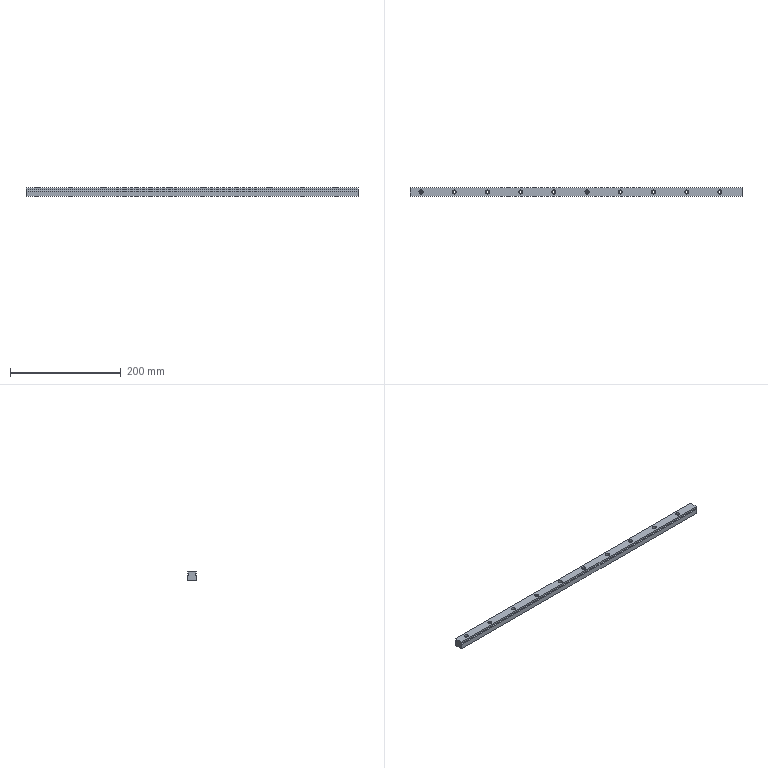Part | SolidWorks | features BaseBody 1 | 1 solid | 60 faces | box 600 x 15 x 15 mm | volume 128298 mm3 | cylinder 42 | plane 18 | commonest cylinder face diameters 4.5 x20 7.5 x20 2.6 x2